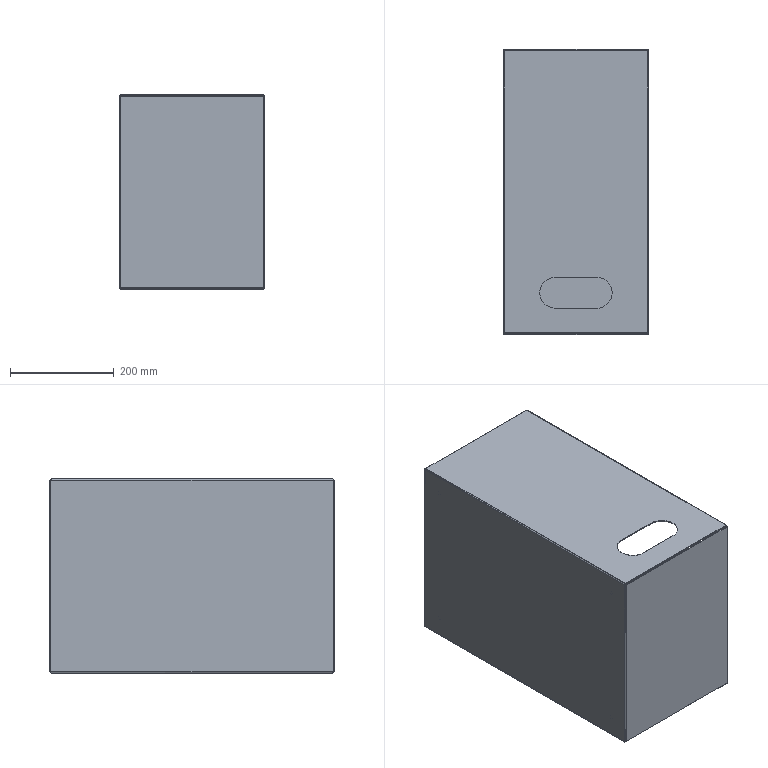Part | SolidWorks | features EdgeFlange 3, Cut 2, ICE 2, FlatPattern 1, SMBaseFlange 1, SheetMetal 1 | 1 solid | 145 faces | box 280 x 550 x 375 mm | volume 1500935 mm3 | plane 92 | cylinder 37 | spline 16 | commonest cylinder face diameters 0.6 x12 4.6 x12 6.8 x8 60 x3 30 x2